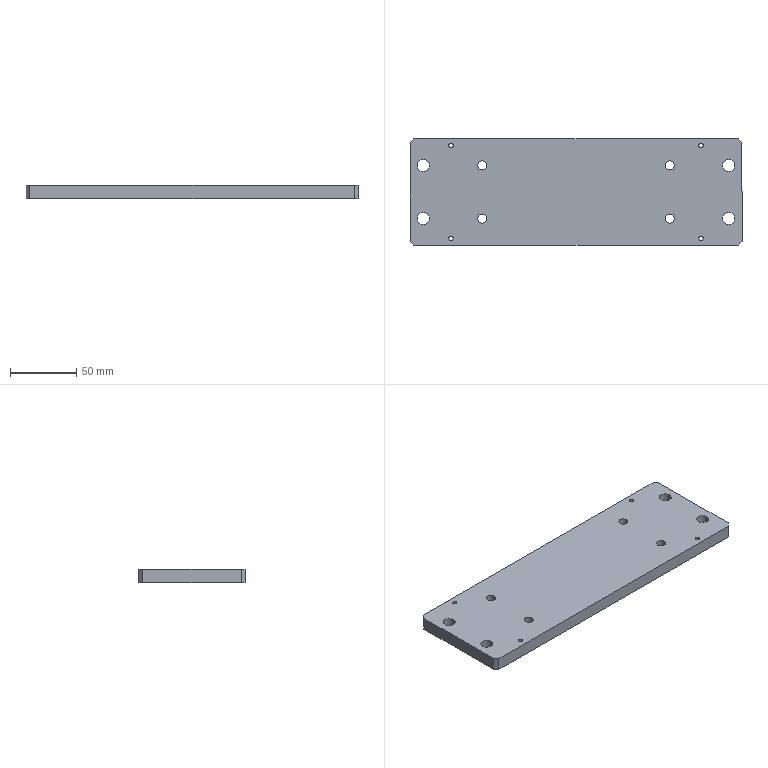Part | SolidWorks | features HoleWzd 3, MirrorPattern 3, Chamfer 1, Extrusion 1 | 1 solid | 34 faces | box 250 x 80 x 10 mm | volume 195481 mm3 | cylinder 24 | plane 10 | commonest cylinder face diameters 3.3 x8 6.8 x8 9 x8
STEP:
#1=CARTESIAN_POINT('',(92.472,75.,0.));
#2=VERTEX_POINT('',#1);
#3=CARTESIAN_POINT('',(95.772,75.,0.));
#4=VERTEX_POINT('',#3);
#5=CARTESIAN_POINT('',(94.122,75.,0.));
#6=DIRECTION('',(0.,0.,1.));
#7=DIRECTION('',(1.,0.,0.));
#8=AXIS2_PLACEMENT_3D('',#5,#6,#7);
#9=CIRCLE('',#8,1.65);
#10=EDGE_CURVE('',#2,#4,#9,.T.);
#11=ORIENTED_EDGE('',*,*,#10,.F.);
#12=CARTESIAN_POINT('',(92.472,75.,10.));
#13=VERTEX_POINT('',#12);
#14=CARTESIAN_POINT('',(92.472,75.,10.));
#15=DIRECTION('',(0.,0.,1.));
#16=VECTOR('',#15,1000.);
#17=LINE('',#14,#16);
#18=EDGE_CURVE('',#2,#13,#17,.T.);
#19=ORIENTED_EDGE('',*,*,#18,.T.);
#20=CARTESIAN_POINT('',(95.772,75.,10.));
#21=VERTEX_POINT('',#20);
#22=CARTESIAN_POINT('',(94.122,75.,10.));
#23=DIRECTION('',(0.,0.,1.));
#24=DIRECTION('',(1.,0.,0.));
#25=AXIS2_PLACEMENT_3D('',#22,#23,#24);
#26=CIRCLE('',#25,1.65);
#27=EDGE_CURVE('',#13,#21,#26,.T.);
#28=ORIENTED_EDGE('',*,*,#27,.T.);
#29=CARTESIAN_POINT('',(95.772,75.,10.));
#30=DIRECTION('',(0.,0.,1.));
#31=VECTOR('',#30,1000.);
#32=LINE('',#29,#31);
#33=EDGE_CURVE('',#4,#21,#32,.T.);
#34=ORIENTED_EDGE('',*,*,#33,.F.);
#35=EDGE_LOOP('',(#11,#19,#28,#34));
#36=FACE_OUTER_BOUND('',#35,.T.);
#37=CARTESIAN_POINT('',(94.122,75.,10.));
#38=DIRECTION('',(0.,0.,1.));
#39=DIRECTION('',(1.,0.,0.));
#40=AXIS2_PLACEMENT_3D('',#37,#38,#39);
#41=CYLINDRICAL_SURFACE('',#40,1.65);
#42=ADVANCED_FACE('',(#36),#41,.F.);
#43=CARTESIAN_POINT('',(92.472,5.,0.));
#44=VERTEX_POINT('',#43);
#45=CARTESIAN_POINT('',(95.772,5.,0.));
#46=VERTEX_POINT('',#45);
#47=CARTESIAN_POINT('',(94.122,5.,0.));
#48=DIRECTION('',(0.,0.,1.));
#49=DIRECTION('',(1.,0.,0.));
#50=AXIS2_PLACEMENT_3D('',#47,#48,#49);
#51=CIRCLE('',#50,1.65);
#52=EDGE_CURVE('',#44,#46,#51,.T.);
#53=ORIENTED_EDGE('',*,*,#52,.F.);
#54=CARTESIAN_POINT('',(92.472,5.,10.));
#55=VERTEX_POINT('',#54);
#56=CARTESIAN_POINT('',(92.472,5.,10.));
#57=DIRECTION('',(0.,0.,1.));
#58=VECTOR('',#57,1000.);
#59=LINE('',#56,#58);
#60=EDGE_CURVE('',#44,#55,#59,.T.);
#61=ORIENTED_EDGE('',*,*,#60,.T.);
#62=CARTESIAN_POINT('',(95.772,5.,10.));
#63=VERTEX_POINT('',#62);
#64=CARTESIAN_POINT('',(94.122,5.,10.));
#65=DIRECTION('',(0.,0.,1.));
#66=DIRECTION('',(1.,0.,0.));
#67=AXIS2_PLACEMENT_3D('',#64,#65,#66);
#68=CIRCLE('',#67,1.65);
#69=EDGE_CURVE('',#55,#63,#68,.T.);
#70=ORIENTED_EDGE('',*,*,#69,.T.);
#71=CARTESIAN_POINT('',(95.772,5.,10.));
#72=DIRECTION('',(0.,0.,1.));
#73=VECTOR('',#72,1000.);
#74=LINE('',#71,#73);
#75=EDGE_CURVE('',#46,#63,#74,.T.);
#76=ORIENTED_EDGE('',*,*,#75,.F.);
#77=EDGE_LOOP('',(#53,#61,#70,#76));
#78=FACE_OUTER_BOUND('',#77,.T.);
#79=CARTESIAN_POINT('',(94.122,5.,10.));
#80=DIRECTION('',(0.,0.,1.));
#81=DIRECTION('',(1.,0.,0.));
#82=AXIS2_PLACEMENT_3D('',#79,#80,#81);
#83=CYLINDRICAL_SURFACE('',#82,1.65);
#84=ADVANCED_FACE('',(#78),#83,.F.);
#85=CARTESIAN_POINT('',(-95.772,75.,0.));
#86=VERTEX_POINT('',#85);
#87=CARTESIAN_POINT('',(-92.472,75.,0.));
#88=VERTEX_POINT('',#87);
#89=CARTESIAN_POINT('',(-94.122,75.,0.));
#90=DIRECTION('',(0.,0.,1.));
#91=DIRECTION('',(1.,0.,0.));
#92=AXIS2_PLACEMENT_3D('',#89,#90,#91);
#93=CIRCLE('',#92,1.65);
#94=EDGE_CURVE('',#86,#88,#93,.T.);
#95=ORIENTED_EDGE('',*,*,#94,.F.);
#96=CARTESIAN_POINT('',(-95.772,75.,10.));
#97=VERTEX_POINT('',#96);
#98=CARTESIAN_POINT('',(-95.772,75.,10.));
#99=DIRECTION('',(0.,0.,1.));
#100=VECTOR('',#99,1000.);
#101=LINE('',#98,#100);
#102=EDGE_CURVE('',#86,#97,#101,.T.);
#103=ORIENTED_EDGE('',*,*,#102,.T.);
#104=CARTESIAN_POINT('',(-92.472,75.,10.));
#105=VERTEX_POINT('',#104);
#106=CARTESIAN_POINT('',(-94.122,75.,10.));
#107=DIRECTION('',(0.,0.,1.));
#108=DIRECTION('',(1.,0.,0.));
#109=AXIS2_PLACEMENT_3D('',#106,#107,#108);
#110=CIRCLE('',#109,1.65);
#111=EDGE_CURVE('',#97,#105,#110,.T.);
#112=ORIENTED_EDGE('',*,*,#111,.T.);
#113=CARTESIAN_POINT('',(-92.472,75.,10.));
#114=DIRECTION('',(0.,0.,1.));
#115=VECTOR('',#114,1000.);
#116=LINE('',#113,#115);
#117=EDGE_CURVE('',#88,#105,#116,.T.);
#118=ORIENTED_EDGE('',*,*,#117,.F.);
#119=EDGE_LOOP('',(#95,#103,#112,#118));
#120=FACE_OUTER_BOUND('',#119,.T.);
#121=CARTESIAN_POINT('',(-94.122,75.,10.));
#122=DIRECTION('',(0.,0.,1.));
#123=DIRECTION('',(1.,0.,0.));
#124=AXIS2_PLACEMENT_3D('',#121,#122,#123);
#125=CYLINDRICAL_SURFACE('',#124,1.65);
#126=ADVANCED_FACE('',(#120),#125,.F.);
#127=CARTESIAN_POINT('',(-95.772,5.,0.));
#128=VERTEX_POINT('',#127);
#129=CARTESIAN_POINT('',(-92.472,5.,0.));
#130=VERTEX_POINT('',#129);
#131=CARTESIAN_POINT('',(-94.122,5.,0.));
#132=DIRECTION('',(0.,0.,1.));
#133=DIRECTION('',(1.,0.,0.));
#134=AXIS2_PLACEMENT_3D('',#131,#132,#133);
#135=CIRCLE('',#134,1.65);
#136=EDGE_CURVE('',#128,#130,#135,.T.);
#137=ORIENTED_EDGE('',*,*,#136,.F.);
#138=CARTESIAN_POINT('',(-95.772,5.,10.));
#139=VERTEX_POINT('',#138);
#140=CARTESIAN_POINT('',(-95.772,5.,10.));
#141=DIRECTION('',(0.,0.,1.));
#142=VECTOR('',#141,1000.);
#143=LINE('',#140,#142);
#144=EDGE_CURVE('',#128,#139,#143,.T.);
#145=ORIENTED_EDGE('',*,*,#144,.T.);
#146=CARTESIAN_POINT('',(-92.472,5.,10.));
#147=VERTEX_POINT('',#146);
#148=CARTESIAN_POINT('',(-94.122,5.,10.));
#149=DIRECTION('',(0.,0.,1.));
#150=DIRECTION('',(1.,0.,0.));
#151=AXIS2_PLACEMENT_3D('',#148,#149,#150);
#152=CIRCLE('',#151,1.65);
#153=EDGE_CURVE('',#139,#147,#152,.T.);
#154=ORIENTED_EDGE('',*,*,#153,.T.);
#155=CARTESIAN_POINT('',(-92.472,5.,10.));
#156=DIRECTION('',(0.,0.,1.));
#157=VECTOR('',#156,1000.);
#158=LINE('',#155,#157);
#159=EDGE_CURVE('',#130,#147,#158,.T.);
#160=ORIENTED_EDGE('',*,*,#159,.F.);
#161=EDGE_LOOP('',(#137,#145,#154,#160));
#162=FACE_OUTER_BOUND('',#161,.T.);
#163=CARTESIAN_POINT('',(-94.122,5.,10.));
#164=DIRECTION('',(0.,0.,1.));
#165=DIRECTION('',(1.,0.,0.));
#166=AXIS2_PLACEMENT_3D('',#163,#164,#165);
#167=CYLINDRICAL_SURFACE('',#166,1.65);
#168=ADVANCED_FACE('',(#162),#167,.F.);
#169=CARTESIAN_POINT('',(-73.9,60.,0.));
#170=VERTEX_POINT('',#169);
#171=CARTESIAN_POINT('',(-67.1,60.,0.));
#172=VERTEX_POINT('',#171);
#173=CARTESIAN_POINT('',(-70.5,60.,0.));
#174=DIRECTION('',(0.,0.,1.));
#175=DIRECTION('',(1.,0.,0.));
#176=AXIS2_PLACEMENT_3D('',#173,#174,#175);
#177=CIRCLE('',#176,3.4);
#178=EDGE_CURVE('',#170,#172,#177,.T.);
#179=ORIENTED_EDGE('',*,*,#178,.F.);
#180=CARTESIAN_POINT('',(-73.9,60.,10.));
#181=VERTEX_POINT('',#180);
#182=CARTESIAN_POINT('',(-73.9,60.,10.));
#183=DIRECTION('',(0.,0.,1.));
#184=VECTOR('',#183,1000.);
#185=LINE('',#182,#184);
#186=EDGE_CURVE('',#170,#181,#185,.T.);
#187=ORIENTED_EDGE('',*,*,#186,.T.);
#188=CARTESIAN_POINT('',(-67.1,60.,10.));
#189=VERTEX_POINT('',#188);
#190=CARTESIAN_POINT('',(-70.5,60.,10.));
#191=DIRECTION('',(0.,0.,1.));
#192=DIRECTION('',(1.,0.,0.));
#193=AXIS2_PLACEMENT_3D('',#190,#191,#192);
#194=CIRCLE('',#193,3.4);
#195=EDGE_CURVE('',#181,#189,#194,.T.);
#196=ORIENTED_EDGE('',*,*,#195,.T.);
#197=CARTESIAN_POINT('',(-67.1,60.,10.));
#198=DIRECTION('',(0.,0.,1.));
#199=VECTOR('',#198,1000.);
#200=LINE('',#197,#199);
#201=EDGE_CURVE('',#172,#189,#200,.T.);
#202=ORIENTED_EDGE('',*,*,#201,.F.);
#203=EDGE_LOOP('',(#179,#187,#196,#202));
#204=FACE_OUTER_BOUND('',#203,.T.);
#205=CARTESIAN_POINT('',(-70.5,60.,10.));
#206=DIRECTION('',(0.,0.,1.));
#207=DIRECTION('',(1.,0.,0.));
#208=AXIS2_PLACEMENT_3D('',#205,#206,#207);
#209=CYLINDRICAL_SURFACE('',#208,3.4);
#210=ADVANCED_FACE('',(#204),#209,.F.);
#211=CARTESIAN_POINT('',(-73.9,20.,0.));
#212=VERTEX_POINT('',#211);
#213=CARTESIAN_POINT('',(-67.1,20.,0.));
#214=VERTEX_POINT('',#213);
#215=CARTESIAN_POINT('',(-70.5,20.,0.));
#216=DIRECTION('',(0.,0.,1.));
#217=DIRECTION('',(1.,0.,0.));
#218=AXIS2_PLACEMENT_3D('',#215,#216,#217);
#219=CIRCLE('',#218,3.4);
#220=EDGE_CURVE('',#212,#214,#219,.T.);
#221=ORIENTED_EDGE('',*,*,#220,.F.);
#222=CARTESIAN_POINT('',(-73.9,20.,10.));
#223=VERTEX_POINT('',#222);
#224=CARTESIAN_POINT('',(-73.9,20.,10.));
#225=DIRECTION('',(0.,0.,1.));
#226=VECTOR('',#225,1000.);
#227=LINE('',#224,#226);
#228=EDGE_CURVE('',#212,#223,#227,.T.);
#229=ORIENTED_EDGE('',*,*,#228,.T.);
#230=CARTESIAN_POINT('',(-67.1,20.,10.));
#231=VERTEX_POINT('',#230);
#232=CARTESIAN_POINT('',(-70.5,20.,10.));
#233=DIRECTION('',(0.,0.,1.));
#234=DIRECTION('',(1.,0.,0.));
#235=AXIS2_PLACEMENT_3D('',#232,#233,#234);
#236=CIRCLE('',#235,3.4);
#237=EDGE_CURVE('',#223,#231,#236,.T.);
#238=ORIENTED_EDGE('',*,*,#237,.T.);
#239=CARTESIAN_POINT('',(-67.1,20.,10.));
#240=DIRECTION('',(0.,0.,1.));
#241=VECTOR('',#240,1000.);
#242=LINE('',#239,#241);
#243=EDGE_CURVE('',#214,#231,#242,.T.);
#244=ORIENTED_EDGE('',*,*,#243,.F.);
#245=EDGE_LOOP('',(#221,#229,#238,#244));
#246=FACE_OUTER_BOUND('',#245,.T.);
#247=CARTESIAN_POINT('',(-70.5,20.,10.));
#248=DIRECTION('',(0.,0.,1.));
#249=DIRECTION('',(1.,0.,0.));
#250=AXIS2_PLACEMENT_3D('',#247,#248,#249);
#251=CYLINDRICAL_SURFACE('',#250,3.4);
#252=ADVANCED_FACE('',(#246),#251,.F.);
#253=CARTESIAN_POINT('',(67.1,60.,0.));
#254=VERTEX_POINT('',#253);
#255=CARTESIAN_POINT('',(73.9,60.,0.));
#256=VERTEX_POINT('',#255);
#257=CARTESIAN_POINT('',(70.5,60.,0.));
#258=DIRECTION('',(0.,0.,1.));
#259=DIRECTION('',(1.,0.,0.));
#260=AXIS2_PLACEMENT_3D('',#257,#258,#259);
#261=CIRCLE('',#260,3.4);
#262=EDGE_CURVE('',#254,#256,#261,.T.);
#263=ORIENTED_EDGE('',*,*,#262,.F.);
#264=CARTESIAN_POINT('',(67.1,60.,10.));
#265=VERTEX_POINT('',#264);
#266=CARTESIAN_POINT('',(67.1,60.,10.));
#267=DIRECTION('',(0.,0.,1.));
#268=VECTOR('',#267,1000.);
#269=LINE('',#266,#268);
#270=EDGE_CURVE('',#254,#265,#269,.T.);
#271=ORIENTED_EDGE('',*,*,#270,.T.);
#272=CARTESIAN_POINT('',(73.9,60.,10.));
#273=VERTEX_POINT('',#272);
#274=CARTESIAN_POINT('',(70.5,60.,10.));
#275=DIRECTION('',(0.,0.,1.));
#276=DIRECTION('',(1.,0.,0.));
#277=AXIS2_PLACEMENT_3D('',#274,#275,#276);
#278=CIRCLE('',#277,3.4);
#279=EDGE_CURVE('',#265,#273,#278,.T.);
#280=ORIENTED_EDGE('',*,*,#279,.T.);
#281=CARTESIAN_POINT('',(73.9,60.,10.));
#282=DIRECTION('',(0.,0.,1.));
#283=VECTOR('',#282,1000.);
#284=LINE('',#281,#283);
#285=EDGE_CURVE('',#256,#273,#284,.T.);
#286=ORIENTED_EDGE('',*,*,#285,.F.);
#287=EDGE_LOOP('',(#263,#271,#280,#286));
#288=FACE_OUTER_BOUND('',#287,.T.);
#289=CARTESIAN_POINT('',(70.5,60.,10.));
#290=DIRECTION('',(0.,0.,1.));
#291=DIRECTION('',(1.,0.,0.));
#292=AXIS2_PLACEMENT_3D('',#289,#290,#291);
#293=CYLINDRICAL_SURFACE('',#292,3.4);
#294=ADVANCED_FACE('',(#288),#293,.F.);
#295=CARTESIAN_POINT('',(67.1,20.,0.));
#296=VERTEX_POINT('',#295);
#297=CARTESIAN_POINT('',(73.9,20.,0.));
#298=VERTEX_POINT('',#297);
#299=CARTESIAN_POINT('',(70.5,20.,0.));
#300=DIRECTION('',(0.,0.,1.));
#301=DIRECTION('',(1.,0.,0.));
#302=AXIS2_PLACEMENT_3D('',#299,#300,#301);
#303=CIRCLE('',#302,3.4);
#304=EDGE_CURVE('',#296,#298,#303,.T.);
#305=ORIENTED_EDGE('',*,*,#304,.F.);
#306=CARTESIAN_POINT('',(67.1,20.,10.));
#307=VERTEX_POINT('',#306);
#308=CARTESIAN_POINT('',(67.1,20.,10.));
#309=DIRECTION('',(0.,0.,1.));
#310=VECTOR('',#309,1000.);
#311=LINE('',#308,#310);
#312=EDGE_CURVE('',#296,#307,#311,.T.);
#313=ORIENTED_EDGE('',*,*,#312,.T.);
#314=CARTESIAN_POINT('',(73.9,20.,10.));
#315=VERTEX_POINT('',#314);
#316=CARTESIAN_POINT('',(70.5,20.,10.));
#317=DIRECTION('',(0.,0.,1.));
#318=DIRECTION('',(1.,0.,0.));
#319=AXIS2_PLACEMENT_3D('',#316,#317,#318);
#320=CIRCLE('',#319,3.4);
#321=EDGE_CURVE('',#307,#315,#320,.T.);
#322=ORIENTED_EDGE('',*,*,#321,.T.);
#323=CARTESIAN_POINT('',(73.9,20.,10.));
#324=DIRECTION('',(0.,0.,1.));
#325=VECTOR('',#324,1000.);
#326=LINE('',#323,#325);
#327=EDGE_CURVE('',#298,#315,#326,.T.);
#328=ORIENTED_EDGE('',*,*,#327,.F.);
#329=EDGE_LOOP('',(#305,#313,#322,#328));
#330=FACE_OUTER_BOUND('',#329,.T.);
#331=CARTESIAN_POINT('',(70.5,20.,10.));
#332=DIRECTION('',(0.,0.,1.));
#333=DIRECTION('',(1.,0.,0.));
#334=AXIS2_PLACEMENT_3D('',#331,#332,#333);
#335=CYLINDRICAL_SURFACE('',#334,3.4);
#336=ADVANCED_FACE('',(#330),#335,.F.);
#337=CARTESIAN_POINT('',(-119.5,20.,0.));
#338=VERTEX_POINT('',#337);
#339=CARTESIAN_POINT('',(-110.5,20.,0.));
#340=VERTEX_POINT('',#339);
#341=CARTESIAN_POINT('',(-115.,20.,0.));
#342=DIRECTION('',(0.,0.,1.));
#343=DIRECTION('',(1.,0.,0.));
#344=AXIS2_PLACEMENT_3D('',#341,#342,#343);
#345=CIRCLE('',#344,4.5);
#346=EDGE_CURVE('',#338,#340,#345,.T.);
#347=ORIENTED_EDGE('',*,*,#346,.F.);
#348=CARTESIAN_POINT('',(-119.5,20.,10.));
#349=VERTEX_POINT('',#348);
#350=CARTESIAN_POINT('',(-119.5,20.,10.));
#351=DIRECTION('',(0.,0.,1.));
#352=VECTOR('',#351,1000.);
#353=LINE('',#350,#352);
#354=EDGE_CURVE('',#338,#349,#353,.T.);
#355=ORIENTED_EDGE('',*,*,#354,.T.);
#356=CARTESIAN_POINT('',(-110.5,20.,10.));
#357=VERTEX_POINT('',#356);
#358=CARTESIAN_POINT('',(-115.,20.,10.));
#359=DIRECTION('',(0.,0.,1.));
#360=DIRECTION('',(1.,0.,0.));
#361=AXIS2_PLACEMENT_3D('',#358,#359,#360);
#362=CIRCLE('',#361,4.5);
#363=EDGE_CURVE('',#349,#357,#362,.T.);
#364=ORIENTED_EDGE('',*,*,#363,.T.);
#365=CARTESIAN_POINT('',(-110.5,20.,10.));
#366=DIRECTION('',(0.,0.,1.));
#367=VECTOR('',#366,1000.);
#368=LINE('',#365,#367);
#369=EDGE_CURVE('',#340,#357,#368,.T.);
#370=ORIENTED_EDGE('',*,*,#369,.F.);
#371=EDGE_LOOP('',(#347,#355,#364,#370));
#372=FACE_OUTER_BOUND('',#371,.T.);
#373=CARTESIAN_POINT('',(-115.,20.,10.));
#374=DIRECTION('',(0.,0.,1.));
#375=DIRECTION('',(1.,0.,0.));
#376=AXIS2_PLACEMENT_3D('',#373,#374,#375);
#377=CYLINDRICAL_SURFACE('',#376,4.5);
#378=ADVANCED_FACE('',(#372),#377,.F.);
#379=CARTESIAN_POINT('',(-119.5,60.,0.));
#380=VERTEX_POINT('',#379);
#381=CARTESIAN_POINT('',(-110.5,60.,0.));
#382=VERTEX_POINT('',#381);
#383=CARTESIAN_POINT('',(-115.,60.,0.));
#384=DIRECTION('',(0.,0.,1.));
#385=DIRECTION('',(1.,0.,0.));
#386=AXIS2_PLACEMENT_3D('',#383,#384,#385);
#387=CIRCLE('',#386,4.5);
#388=EDGE_CURVE('',#380,#382,#387,.T.);
#389=ORIENTED_EDGE('',*,*,#388,.F.);
#390=CARTESIAN_POINT('',(-119.5,60.,10.));
#391=VERTEX_POINT('',#390);
#392=CARTESIAN_POINT('',(-119.5,60.,10.));
#393=DIRECTION('',(0.,0.,1.));
#394=VECTOR('',#393,1000.);
#395=LINE('',#392,#394);
#396=EDGE_CURVE('',#380,#391,#395,.T.);
#397=ORIENTED_EDGE('',*,*,#396,.T.);
#398=CARTESIAN_POINT('',(-110.5,60.,10.));
#399=VERTEX_POINT('',#398);
#400=CARTESIAN_POINT('',(-115.,60.,10.));
#401=DIRECTION('',(0.,0.,1.));
#402=DIRECTION('',(1.,0.,0.));
#403=AXIS2_PLACEMENT_3D('',#400,#401,#402);
#404=CIRCLE('',#403,4.5);
#405=EDGE_CURVE('',#391,#399,#404,.T.);
#406=ORIENTED_EDGE('',*,*,#405,.T.);
#407=CARTESIAN_POINT('',(-110.5,60.,10.));
#408=DIRECTION('',(0.,0.,1.));
#409=VECTOR('',#408,1000.);
#410=LINE('',#407,#409);
#411=EDGE_CURVE('',#382,#399,#410,.T.);
#412=ORIENTED_EDGE('',*,*,#411,.F.);
#413=EDGE_LOOP('',(#389,#397,#406,#412));
#414=FACE_OUTER_BOUND('',#413,.T.);
#415=CARTESIAN_POINT('',(-115.,60.,10.));
#416=DIRECTION('',(0.,0.,1.));
#417=DIRECTION('',(1.,0.,0.));
#418=AXIS2_PLACEMENT_3D('',#415,#416,#417);
#419=CYLINDRICAL_SURFACE('',#418,4.5);
#420=ADVANCED_FACE('',(#414),#419,.F.);
#421=CARTESIAN_POINT('',(110.5,20.,0.));
#422=VERTEX_POINT('',#421);
#423=CARTESIAN_POINT('',(119.5,20.,0.));
#424=VERTEX_POINT('',#423);
#425=CARTESIAN_POINT('',(115.,20.,0.));
#426=DIRECTION('',(0.,0.,1.));
#427=DIRECTION('',(1.,0.,0.));
#428=AXIS2_PLACEMENT_3D('',#425,#426,#427);
#429=CIRCLE('',#428,4.5);
#430=EDGE_CURVE('',#422,#424,#429,.T.);
#431=ORIENTED_EDGE('',*,*,#430,.F.);
#432=CARTESIAN_POINT('',(110.5,20.,10.));
#433=VERTEX_POINT('',#432);
#434=CARTESIAN_POINT('',(110.5,20.,10.));
#435=DIRECTION('',(0.,0.,1.));
#436=VECTOR('',#435,1000.);
#437=LINE('',#434,#436);
#438=EDGE_CURVE('',#422,#433,#437,.T.);
#439=ORIENTED_EDGE('',*,*,#438,.T.);
#440=CARTESIAN_POINT('',(119.5,20.,10.));
#441=VERTEX_POINT('',#440);
#442=CARTESIAN_POINT('',(115.,20.,10.));
#443=DIRECTION('',(0.,0.,1.));
#444=DIRECTION('',(1.,0.,0.));
#445=AXIS2_PLACEMENT_3D('',#442,#443,#444);
#446=CIRCLE('',#445,4.5);
#447=EDGE_CURVE('',#433,#441,#446,.T.);
#448=ORIENTED_EDGE('',*,*,#447,.T.);
#449=CARTESIAN_POINT('',(119.5,20.,10.));
#450=DIRECTION('',(0.,0.,1.));
#451=VECTOR('',#450,1000.);
#452=LINE('',#449,#451);
#453=EDGE_CURVE('',#424,#441,#452,.T.);
#454=ORIENTED_EDGE('',*,*,#453,.F.);
#455=EDGE_LOOP('',(#431,#439,#448,#454));
#456=FACE_OUTER_BOUND('',#455,.T.);
#457=CARTESIAN_POINT('',(115.,20.,10.));
#458=DIRECTION('',(0.,0.,1.));
#459=DIRECTION('',(1.,0.,0.));
#460=AXIS2_PLACEMENT_3D('',#457,#458,#459);
#461=CYLINDRICAL_SURFACE('',#460,4.5);
#462=ADVANCED_FACE('',(#456),#461,.F.);
#463=CARTESIAN_POINT('',(110.5,60.,0.));
#464=VERTEX_POINT('',#463);
#465=CARTESIAN_POINT('',(119.5,60.,0.));
#466=VERTEX_POINT('',#465);
#467=CARTESIAN_POINT('',(115.,60.,0.));
#468=DIRECTION('',(0.,0.,1.));
#469=DIRECTION('',(1.,0.,0.));
#470=AXIS2_PLACEMENT_3D('',#467,#468,#469);
#471=CIRCLE('',#470,4.5);
#472=EDGE_CURVE('',#464,#466,#471,.T.);
#473=ORIENTED_EDGE('',*,*,#472,.F.);
#474=CARTESIAN_POINT('',(110.5,60.,10.));
#475=VERTEX_POINT('',#474);
#476=CARTESIAN_POINT('',(110.5,60.,10.));
#477=DIRECTION('',(0.,0.,1.));
#478=VECTOR('',#477,1000.);
#479=LINE('',#476,#478);
#480=EDGE_CURVE('',#464,#475,#479,.T.);
#481=ORIENTED_EDGE('',*,*,#480,.T.);
#482=CARTESIAN_POINT('',(119.5,60.,10.));
#483=VERTEX_POINT('',#482);
#484=CARTESIAN_POINT('',(115.,60.,10.));
#485=DIRECTION('',(0.,0.,1.));
#486=DIRECTION('',(1.,0.,0.));
#487=AXIS2_PLACEMENT_3D('',#484,#485,#486);
#488=CIRCLE('',#487,4.5);
#489=EDGE_CURVE('',#475,#483,#488,.T.);
#490=ORIENTED_EDGE('',*,*,#489,.T.);
#491=CARTESIAN_POINT('',(119.5,60.,10.));
#492=DIRECTION('',(0.,0.,1.));
#493=VECTOR('',#492,1000.);
#494=LINE('',#491,#493);
#495=EDGE_CURVE('',#466,#483,#494,.T.);
#496=ORIENTED_EDGE('',*,*,#495,.F.);
#497=EDGE_LOOP('',(#473,#481,#490,#496));
#498=FACE_OUTER_BOUND('',#497,.T.);
#499=CARTESIAN_POINT('',(115.,60.,10.));
#500=DIRECTION('',(0.,0.,1.));
#501=DIRECTION('',(1.,0.,0.));
#502=AXIS2_PLACEMENT_3D('',#499,#500,#501);
#503=CYLINDRICAL_SURFACE('',#502,4.5);
#504=ADVANCED_FACE('',(#498),#503,.F.);
#505=CARTESIAN_POINT('',(-125.,77.,10.));
#506=VERTEX_POINT('',#505);
#507=CARTESIAN_POINT('',(-125.,3.,10.));
#508=VERTEX_POINT('',#507);
#509=CARTESIAN_POINT('',(-125.,80.,10.));
#510=DIRECTION('',(0.,-1.,0.));
#511=VECTOR('',#510,1000.);
#512=LINE('',#509,#511);
#513=EDGE_CURVE('',#506,#508,#512,.T.);
#514=ORIENTED_EDGE('',*,*,#513,.F.);
#515=CARTESIAN_POINT('',(-125.,77.,0.));
#516=VERTEX_POINT('',#515);
#517=CARTESIAN_POINT('',(-125.,77.,10.));
#518=DIRECTION('',(0.,0.,-1.));
#519=VECTOR('',#518,1000.);
#520=LINE('',#517,#519);
#521=EDGE_CURVE('',#506,#516,#520,.T.);
#522=ORIENTED_EDGE('',*,*,#521,.T.);
#523=CARTESIAN_POINT('',(-125.,3.,0.));
#524=VERTEX_POINT('',#523);
#525=CARTESIAN_POINT('',(-125.,80.,0.));
#526=DIRECTION('',(0.,-1.,0.));
#527=VECTOR('',#526,1000.);
#528=LINE('',#525,#527);
#529=EDGE_CURVE('',#516,#524,#528,.T.);
#530=ORIENTED_EDGE('',*,*,#529,.T.);
#531=CARTESIAN_POINT('',(-125.,3.,10.));
#532=DIRECTION('',(0.,0.,1.));
#533=VECTOR('',#532,1000.);
#534=LINE('',#531,#533);
#535=EDGE_CURVE('',#524,#508,#534,.T.);
#536=ORIENTED_EDGE('',*,*,#535,.T.);
#537=EDGE_LOOP('',(#514,#522,#530,#536));
#538=FACE_OUTER_BOUND('',#537,.T.);
#539=CARTESIAN_POINT('',(-125.,80.,10.));
#540=DIRECTION('',(1.,0.,0.));
#541=DIRECTION('',(0.,1.,0.));
#542=AXIS2_PLACEMENT_3D('',#539,#540,#541);
#543=PLANE('',#542);
#544=ADVANCED_FACE('',(#538),#543,.F.);
#545=CARTESIAN_POINT('',(-122.,0.,10.));
#546=VERTEX_POINT('',#545);
#547=CARTESIAN_POINT('',(122.,0.,10.));
#548=VERTEX_POINT('',#547);
#549=CARTESIAN_POINT('',(-125.,0.,10.));
#550=DIRECTION('',(1.,0.,0.));
#551=VECTOR('',#550,1000.);
#552=LINE('',#549,#551);
#553=EDGE_CURVE('',#546,#548,#552,.T.);
#554=ORIENTED_EDGE('',*,*,#553,.F.);
#555=CARTESIAN_POINT('',(-122.,0.,0.));
#556=VERTEX_POINT('',#555);
#557=CARTESIAN_POINT('',(-122.,0.,10.));
#558=DIRECTION('',(0.,0.,-1.));
#559=VECTOR('',#558,1000.);
#560=LINE('',#557,#559);
#561=EDGE_CURVE('',#546,#556,#560,.T.);
#562=ORIENTED_EDGE('',*,*,#561,.T.);
#563=CARTESIAN_POINT('',(122.,0.,0.));
#564=VERTEX_POINT('',#563);
#565=CARTESIAN_POINT('',(-125.,0.,0.));
#566=DIRECTION('',(1.,0.,0.));
#567=VECTOR('',#566,1000.);
#568=LINE('',#565,#567);
#569=EDGE_CURVE('',#556,#564,#568,.T.);
#570=ORIENTED_EDGE('',*,*,#569,.T.);
#571=CARTESIAN_POINT('',(122.,0.,10.));
#572=DIRECTION('',(0.,0.,1.));
#573=VECTOR('',#572,1000.);
#574=LINE('',#571,#573);
#575=EDGE_CURVE('',#564,#548,#574,.T.);
#576=ORIENTED_EDGE('',*,*,#575,.T.);
#577=EDGE_LOOP('',(#554,#562,#570,#576));
#578=FACE_OUTER_BOUND('',#577,.T.);
#579=CARTESIAN_POINT('',(-125.,0.,10.));
#580=DIRECTION('',(0.,1.,0.));
#581=DIRECTION('',(0.,0.,1.));
#582=AXIS2_PLACEMENT_3D('',#579,#580,#581);
#583=PLANE('',#582);
#584=ADVANCED_FACE('',(#578),#583,.F.);
#585=CARTESIAN_POINT('',(125.,3.,10.));
#586=VERTEX_POINT('',#585);
#587=CARTESIAN_POINT('',(125.,77.,10.));
#588=VERTEX_POINT('',#587);
#589=CARTESIAN_POINT('',(125.,80.,10.));
#590=DIRECTION('',(0.,1.,0.));
#591=VECTOR('',#590,1000.);
#592=LINE('',#589,#591);
#593=EDGE_CURVE('',#586,#588,#592,.T.);
#594=ORIENTED_EDGE('',*,*,#593,.F.);
#595=CARTESIAN_POINT('',(125.,3.,0.));
#596=VERTEX_POINT('',#595);
#597=CARTESIAN_POINT('',(125.,3.,10.));
#598=DIRECTION('',(0.,0.,-1.));
#599=VECTOR('',#598,1000.);
#600=LINE('',#597,#599);
#601=EDGE_CURVE('',#586,#596,#600,.T.);
#602=ORIENTED_EDGE('',*,*,#601,.T.);
#603=CARTESIAN_POINT('',(125.,77.,0.));
#604=VERTEX_POINT('',#603);
#605=CARTESIAN_POINT('',(125.,80.,0.));
#606=DIRECTION('',(0.,1.,0.));
#607=VECTOR('',#606,1000.);
#608=LINE('',#605,#607);
#609=EDGE_CURVE('',#596,#604,#608,.T.);
#610=ORIENTED_EDGE('',*,*,#609,.T.);
#611=CARTESIAN_POINT('',(125.,77.,10.));
#612=DIRECTION('',(0.,0.,1.));
#613=VECTOR('',#612,1000.);
#614=LINE('',#611,#613);
#615=EDGE_CURVE('',#604,#588,#614,.T.);
#616=ORIENTED_EDGE('',*,*,#615,.T.);
#617=EDGE_LOOP('',(#594,#602,#610,#616));
#618=FACE_OUTER_BOUND('',#617,.T.);
#619=CARTESIAN_POINT('',(125.,80.,10.));
#620=DIRECTION('',(-1.,0.,0.));
#621=DIRECTION('',(0.,-1.,0.));
#622=AXIS2_PLACEMENT_3D('',#619,#620,#621);
#623=PLANE('',#622);
#624=ADVANCED_FACE('',(#618),#623,.F.);
#625=CARTESIAN_POINT('',(122.,80.,0.));
#626=VERTEX_POINT('',#625);
#627=CARTESIAN_POINT('',(-122.,80.,0.));
#628=VERTEX_POINT('',#627);
#629=CARTESIAN_POINT('',(-125.,80.,0.));
#630=DIRECTION('',(-1.,0.,0.));
#631=VECTOR('',#630,1000.);
#632=LINE('',#629,#631);
#633=EDGE_CURVE('',#626,#628,#632,.T.);
#634=ORIENTED_EDGE('',*,*,#633,.T.);
#635=CARTESIAN_POINT('',(-122.,80.,10.));
#636=VERTEX_POINT('',#635);
#637=CARTESIAN_POINT('',(-122.,80.,10.));
#638=DIRECTION('',(0.,0.,1.));
#639=VECTOR('',#638,1000.);
#640=LINE('',#637,#639);
#641=EDGE_CURVE('',#628,#636,#640,.T.);
#642=ORIENTED_EDGE('',*,*,#641,.T.);
#643=CARTESIAN_POINT('',(122.,80.,10.));
#644=VERTEX_POINT('',#643);
#645=CARTESIAN_POINT('',(-125.,80.,10.));
#646=DIRECTION('',(-1.,0.,0.));
#647=VECTOR('',#646,1000.);
#648=LINE('',#645,#647);
#649=EDGE_CURVE('',#644,#636,#648,.T.);
#650=ORIENTED_EDGE('',*,*,#649,.F.);
#651=CARTESIAN_POINT('',(122.,80.,10.));
#652=DIRECTION('',(0.,0.,-1.));
#653=VECTOR('',#652,1000.);
#654=LINE('',#651,#653);
#655=EDGE_CURVE('',#644,#626,#654,.T.);
#656=ORIENTED_EDGE('',*,*,#655,.T.);
#657=EDGE_LOOP('',(#634,#642,#650,#656));
#658=FACE_OUTER_BOUND('',#657,.T.);
#659=CARTESIAN_POINT('',(-125.,80.,10.));
#660=DIRECTION('',(0.,-1.,0.));
#661=DIRECTION('',(0.,0.,-1.));
#662=AXIS2_PLACEMENT_3D('',#659,#660,#661);
#663=PLANE('',#662);
#664=ADVANCED_FACE('',(#658),#663,.F.);
#665=CARTESIAN_POINT('',(94.122,75.,10.));
#666=DIRECTION('',(0.,0.,1.));
#667=DIRECTION('',(1.,0.,0.));
#668=AXIS2_PLACEMENT_3D('',#665,#666,#667);
#669=CIRCLE('',#668,1.65);
#670=EDGE_CURVE('',#21,#13,#669,.T.);
#671=ORIENTED_EDGE('',*,*,#670,.F.);
#672=ORIENTED_EDGE('',*,*,#27,.F.);
#673=EDGE_LOOP('',(#671,#672));
#674=FACE_BOUND('',#673,.T.);
#675=CARTESIAN_POINT('',(94.122,5.,10.));
#676=DIRECTION('',(0.,0.,1.));
#677=DIRECTION('',(1.,0.,0.));
#678=AXIS2_PLACEMENT_3D('',#675,#676,#677);
#679=CIRCLE('',#678,1.65);
#680=EDGE_CURVE('',#63,#55,#679,.T.);
#681=ORIENTED_EDGE('',*,*,#680,.F.);
#682=ORIENTED_EDGE('',*,*,#69,.F.);
#683=EDGE_LOOP('',(#681,#682));
#684=FACE_BOUND('',#683,.T.);
#685=CARTESIAN_POINT('',(-94.122,75.,10.));
#686=DIRECTION('',(0.,0.,1.));
#687=DIRECTION('',(1.,0.,0.));
#688=AXIS2_PLACEMENT_3D('',#685,#686,#687);
#689=CIRCLE('',#688,1.65);
#690=EDGE_CURVE('',#105,#97,#689,.T.);
#691=ORIENTED_EDGE('',*,*,#690,.F.);
#692=ORIENTED_EDGE('',*,*,#111,.F.);
#693=EDGE_LOOP('',(#691,#692));
#694=FACE_BOUND('',#693,.T.);
#695=CARTESIAN_POINT('',(-94.122,5.,10.));
#696=DIRECTION('',(0.,0.,1.));
#697=DIRECTION('',(1.,0.,0.));
#698=AXIS2_PLACEMENT_3D('',#695,#696,#697);
#699=CIRCLE('',#698,1.65);
#700=EDGE_CURVE('',#147,#139,#699,.T.);
#701=ORIENTED_EDGE('',*,*,#700,.F.);
#702=ORIENTED_EDGE('',*,*,#153,.F.);
#703=EDGE_LOOP('',(#701,#702));
#704=FACE_BOUND('',#703,.T.);
#705=CARTESIAN_POINT('',(-70.5,60.,10.));
#706=DIRECTION('',(0.,0.,1.));
#707=DIRECTION('',(1.,0.,0.));
#708=AXIS2_PLACEMENT_3D('',#705,#706,#707);
#709=CIRCLE('',#708,3.4);
#710=EDGE_CURVE('',#189,#181,#709,.T.);
#711=ORIENTED_EDGE('',*,*,#710,.F.);
#712=ORIENTED_EDGE('',*,*,#195,.F.);
#713=EDGE_LOOP('',(#711,#712));
#714=FACE_BOUND('',#713,.T.);
#715=CARTESIAN_POINT('',(-70.5,20.,10.));
#716=DIRECTION('',(0.,0.,1.));
#717=DIRECTION('',(1.,0.,0.));
#718=AXIS2_PLACEMENT_3D('',#715,#716,#717);
#719=CIRCLE('',#718,3.4);
#720=EDGE_CURVE('',#231,#223,#719,.T.);
#721=ORIENTED_EDGE('',*,*,#720,.F.);
#722=ORIENTED_EDGE('',*,*,#237,.F.);
#723=EDGE_LOOP('',(#721,#722));
#724=FACE_BOUND('',#723,.T.);
#725=CARTESIAN_POINT('',(70.5,60.,10.));
#726=DIRECTION('',(0.,0.,1.));
#727=DIRECTION('',(1.,0.,0.));
#728=AXIS2_PLACEMENT_3D('',#725,#726,#727);
#729=CIRCLE('',#728,3.4);
#730=EDGE_CURVE('',#273,#265,#729,.T.);
#731=ORIENTED_EDGE('',*,*,#730,.F.);
#732=ORIENTED_EDGE('',*,*,#279,.F.);
#733=EDGE_LOOP('',(#731,#732));
#734=FACE_BOUND('',#733,.T.);
#735=CARTESIAN_POINT('',(70.5,20.,10.));
#736=DIRECTION('',(0.,0.,1.));
#737=DIRECTION('',(1.,0.,0.));
#738=AXIS2_PLACEMENT_3D('',#735,#736,#737);
#739=CIRCLE('',#738,3.4);
#740=EDGE_CURVE('',#315,#307,#739,.T.);
#741=ORIENTED_EDGE('',*,*,#740,.F.);
#742=ORIENTED_EDGE('',*,*,#321,.F.);
#743=EDGE_LOOP('',(#741,#742));
#744=FACE_BOUND('',#743,.T.);
#745=CARTESIAN_POINT('',(-115.,20.,10.));
#746=DIRECTION('',(0.,0.,1.));
#747=DIRECTION('',(1.,0.,0.));
#748=AXIS2_PLACEMENT_3D('',#745,#746,#747);
#749=CIRCLE('',#748,4.5);
#750=EDGE_CURVE('',#357,#349,#749,.T.);
#751=ORIENTED_EDGE('',*,*,#750,.F.);
#752=ORIENTED_EDGE('',*,*,#363,.F.);
#753=EDGE_LOOP('',(#751,#752));
#754=FACE_BOUND('',#753,.T.);
#755=CARTESIAN_POINT('',(-115.,60.,10.));
#756=DIRECTION('',(0.,0.,1.));
#757=DIRECTION('',(1.,0.,0.));
#758=AXIS2_PLACEMENT_3D('',#755,#756,#757);
#759=CIRCLE('',#758,4.5);
#760=EDGE_CURVE('',#399,#391,#759,.T.);
#761=ORIENTED_EDGE('',*,*,#760,.F.);
#762=ORIENTED_EDGE('',*,*,#405,.F.);
#763=EDGE_LOOP('',(#761,#762));
#764=FACE_BOUND('',#763,.T.);
#765=CARTESIAN_POINT('',(115.,20.,10.));
#766=DIRECTION('',(0.,0.,1.));
#767=DIRECTION('',(1.,0.,0.));
#768=AXIS2_PLACEMENT_3D('',#765,#766,#767);
#769=CIRCLE('',#768,4.5);
#770=EDGE_CURVE('',#441,#433,#769,.T.);
#771=ORIENTED_EDGE('',*,*,#770,.F.);
#772=ORIENTED_EDGE('',*,*,#447,.F.);
#773=EDGE_LOOP('',(#771,#772));
#774=FACE_BOUND('',#773,.T.);
#775=CARTESIAN_POINT('',(115.,60.,10.));
#776=DIRECTION('',(0.,0.,1.));
#777=DIRECTION('',(1.,0.,0.));
#778=AXIS2_PLACEMENT_3D('',#775,#776,#777);
#779=CIRCLE('',#778,4.5);
#780=EDGE_CURVE('',#483,#475,#779,.T.);
#781=ORIENTED_EDGE('',*,*,#780,.F.);
#782=ORIENTED_EDGE('',*,*,#489,.F.);
#783=EDGE_LOOP('',(#781,#782));
#784=FACE_BOUND('',#783,.T.);
#785=ORIENTED_EDGE('',*,*,#649,.T.);
#786=CARTESIAN_POINT('',(-101.,101.,10.));
#787=DIRECTION('',(-0.7071,-0.7071,0.));
#788=VECTOR('',#787,1000.);
#789=LINE('',#786,#788);
#790=EDGE_CURVE('',#636,#506,#789,.T.);
#791=ORIENTED_EDGE('',*,*,#790,.T.);
#792=ORIENTED_EDGE('',*,*,#513,.T.);
#793=CARTESIAN_POINT('',(-61.,-61.,10.));
#794=DIRECTION('',(0.7071,-0.7071,0.));
#795=VECTOR('',#794,1000.);
#796=LINE('',#793,#795);
#797=EDGE_CURVE('',#508,#546,#796,.T.);
#798=ORIENTED_EDGE('',*,*,#797,.T.);
#799=ORIENTED_EDGE('',*,*,#553,.T.);
#800=CARTESIAN_POINT('',(61.,-61.,10.));
#801=DIRECTION('',(0.7071,0.7071,0.));
#802=VECTOR('',#801,1000.);
#803=LINE('',#800,#802);
#804=EDGE_CURVE('',#548,#586,#803,.T.);
#805=ORIENTED_EDGE('',*,*,#804,.T.);
#806=ORIENTED_EDGE('',*,*,#593,.T.);
#807=CARTESIAN_POINT('',(101.,101.,10.));
#808=DIRECTION('',(-0.7071,0.7071,0.));
#809=VECTOR('',#808,1000.);
#810=LINE('',#807,#809);
#811=EDGE_CURVE('',#588,#644,#810,.T.);
#812=ORIENTED_EDGE('',*,*,#811,.T.);
#813=EDGE_LOOP('',(#785,#791,#792,#798,#799,#805,#806,#812));
#814=FACE_OUTER_BOUND('',#813,.T.);
#815=CARTESIAN_POINT('',(0.,0.,10.));
#816=DIRECTION('',(0.,0.,1.));
#817=DIRECTION('',(1.,0.,0.));
#818=AXIS2_PLACEMENT_3D('',#815,#816,#817);
#819=PLANE('',#818);
#820=ADVANCED_FACE('',(#674,#684,#694,#704,#714,#724,#734,#744,#754,#764,#774,#784,#814),#819,.T.);
#821=CARTESIAN_POINT('',(94.122,75.,0.));
#822=DIRECTION('',(0.,0.,1.));
#823=DIRECTION('',(1.,0.,0.));
#824=AXIS2_PLACEMENT_3D('',#821,#822,#823);
#825=CIRCLE('',#824,1.65);
#826=EDGE_CURVE('',#4,#2,#825,.T.);
#827=ORIENTED_EDGE('',*,*,#826,.T.);
#828=ORIENTED_EDGE('',*,*,#10,.T.);
#829=EDGE_LOOP('',(#827,#828));
#830=FACE_BOUND('',#829,.T.);
#831=CARTESIAN_POINT('',(94.122,5.,0.));
#832=DIRECTION('',(0.,0.,1.));
#833=DIRECTION('',(1.,0.,0.));
#834=AXIS2_PLACEMENT_3D('',#831,#832,#833);
#835=CIRCLE('',#834,1.65);
#836=EDGE_CURVE('',#46,#44,#835,.T.);
#837=ORIENTED_EDGE('',*,*,#836,.T.);
#838=ORIENTED_EDGE('',*,*,#52,.T.);
#839=EDGE_LOOP('',(#837,#838));
#840=FACE_BOUND('',#839,.T.);
#841=CARTESIAN_POINT('',(-94.122,75.,0.));
#842=DIRECTION('',(0.,0.,1.));
#843=DIRECTION('',(1.,0.,0.));
#844=AXIS2_PLACEMENT_3D('',#841,#842,#843);
#845=CIRCLE('',#844,1.65);
#846=EDGE_CURVE('',#88,#86,#845,.T.);
#847=ORIENTED_EDGE('',*,*,#846,.T.);
#848=ORIENTED_EDGE('',*,*,#94,.T.);
#849=EDGE_LOOP('',(#847,#848));
#850=FACE_BOUND('',#849,.T.);
#851=CARTESIAN_POINT('',(-94.122,5.,0.));
#852=DIRECTION('',(0.,0.,1.));
#853=DIRECTION('',(1.,0.,0.));
#854=AXIS2_PLACEMENT_3D('',#851,#852,#853);
#855=CIRCLE('',#854,1.65);
#856=EDGE_CURVE('',#130,#128,#855,.T.);
#857=ORIENTED_EDGE('',*,*,#856,.T.);
#858=ORIENTED_EDGE('',*,*,#136,.T.);
#859=EDGE_LOOP('',(#857,#858));
#860=FACE_BOUND('',#859,.T.);
#861=CARTESIAN_POINT('',(-70.5,60.,0.));
#862=DIRECTION('',(0.,0.,1.));
#863=DIRECTION('',(1.,0.,0.));
#864=AXIS2_PLACEMENT_3D('',#861,#862,#863);
#865=CIRCLE('',#864,3.4);
#866=EDGE_CURVE('',#172,#170,#865,.T.);
#867=ORIENTED_EDGE('',*,*,#866,.T.);
#868=ORIENTED_EDGE('',*,*,#178,.T.);
#869=EDGE_LOOP('',(#867,#868));
#870=FACE_BOUND('',#869,.T.);
#871=CARTESIAN_POINT('',(-70.5,20.,0.));
#872=DIRECTION('',(0.,0.,1.));
#873=DIRECTION('',(1.,0.,0.));
#874=AXIS2_PLACEMENT_3D('',#871,#872,#873);
#875=CIRCLE('',#874,3.4);
#876=EDGE_CURVE('',#214,#212,#875,.T.);
#877=ORIENTED_EDGE('',*,*,#876,.T.);
#878=ORIENTED_EDGE('',*,*,#220,.T.);
#879=EDGE_LOOP('',(#877,#878));
#880=FACE_BOUND('',#879,.T.);
#881=CARTESIAN_POINT('',(70.5,60.,0.));
#882=DIRECTION('',(0.,0.,1.));
#883=DIRECTION('',(1.,0.,0.));
#884=AXIS2_PLACEMENT_3D('',#881,#882,#883);
#885=CIRCLE('',#884,3.4);
#886=EDGE_CURVE('',#256,#254,#885,.T.);
#887=ORIENTED_EDGE('',*,*,#886,.T.);
#888=ORIENTED_EDGE('',*,*,#262,.T.);
#889=EDGE_LOOP('',(#887,#888));
#890=FACE_BOUND('',#889,.T.);
#891=CARTESIAN_POINT('',(70.5,20.,0.));
#892=DIRECTION('',(0.,0.,1.));
#893=DIRECTION('',(1.,0.,0.));
#894=AXIS2_PLACEMENT_3D('',#891,#892,#893);
#895=CIRCLE('',#894,3.4);
#896=EDGE_CURVE('',#298,#296,#895,.T.);
#897=ORIENTED_EDGE('',*,*,#896,.T.);
#898=ORIENTED_EDGE('',*,*,#304,.T.);
#899=EDGE_LOOP('',(#897,#898));
#900=FACE_BOUND('',#899,.T.);
#901=CARTESIAN_POINT('',(-115.,20.,0.));
#902=DIRECTION('',(0.,0.,1.));
#903=DIRECTION('',(1.,0.,0.));
#904=AXIS2_PLACEMENT_3D('',#901,#902,#903);
#905=CIRCLE('',#904,4.5);
#906=EDGE_CURVE('',#340,#338,#905,.T.);
#907=ORIENTED_EDGE('',*,*,#906,.T.);
#908=ORIENTED_EDGE('',*,*,#346,.T.);
#909=EDGE_LOOP('',(#907,#908));
#910=FACE_BOUND('',#909,.T.);
#911=CARTESIAN_POINT('',(-115.,60.,0.));
#912=DIRECTION('',(0.,0.,1.));
#913=DIRECTION('',(1.,0.,0.));
#914=AXIS2_PLACEMENT_3D('',#911,#912,#913);
#915=CIRCLE('',#914,4.5);
#916=EDGE_CURVE('',#382,#380,#915,.T.);
#917=ORIENTED_EDGE('',*,*,#916,.T.);
#918=ORIENTED_EDGE('',*,*,#388,.T.);
#919=EDGE_LOOP('',(#917,#918));
#920=FACE_BOUND('',#919,.T.);
#921=CARTESIAN_POINT('',(115.,20.,0.));
#922=DIRECTION('',(0.,0.,1.));
#923=DIRECTION('',(1.,0.,0.));
#924=AXIS2_PLACEMENT_3D('',#921,#922,#923);
#925=CIRCLE('',#924,4.5);
#926=EDGE_CURVE('',#424,#422,#925,.T.);
#927=ORIENTED_EDGE('',*,*,#926,.T.);
#928=ORIENTED_EDGE('',*,*,#430,.T.);
#929=EDGE_LOOP('',(#927,#928));
#930=FACE_BOUND('',#929,.T.);
#931=CARTESIAN_POINT('',(115.,60.,0.));
#932=DIRECTION('',(0.,0.,1.));
#933=DIRECTION('',(1.,0.,0.));
#934=AXIS2_PLACEMENT_3D('',#931,#932,#933);
#935=CIRCLE('',#934,4.5);
#936=EDGE_CURVE('',#466,#464,#935,.T.);
#937=ORIENTED_EDGE('',*,*,#936,.T.);
#938=ORIENTED_EDGE('',*,*,#472,.T.);
#939=EDGE_LOOP('',(#937,#938));
#940=FACE_BOUND('',#939,.T.);
#941=ORIENTED_EDGE('',*,*,#529,.F.);
#942=CARTESIAN_POINT('',(-125.,77.,0.));
#943=DIRECTION('',(0.7071,0.7071,0.));
#944=VECTOR('',#943,1000.);
#945=LINE('',#942,#944);
#946=EDGE_CURVE('',#516,#628,#945,.T.);
#947=ORIENTED_EDGE('',*,*,#946,.T.);
#948=ORIENTED_EDGE('',*,*,#633,.F.);
#949=CARTESIAN_POINT('',(122.,80.,0.));
#950=DIRECTION('',(0.7071,-0.7071,0.));
#951=VECTOR('',#950,1000.);
#952=LINE('',#949,#951);
#953=EDGE_CURVE('',#626,#604,#952,.T.);
#954=ORIENTED_EDGE('',*,*,#953,.T.);
#955=ORIENTED_EDGE('',*,*,#609,.F.);
#956=CARTESIAN_POINT('',(125.,3.,0.));
#957=DIRECTION('',(-0.7071,-0.7071,0.));
#958=VECTOR('',#957,1000.);
#959=LINE('',#956,#958);
#960=EDGE_CURVE('',#596,#564,#959,.T.);
#961=ORIENTED_EDGE('',*,*,#960,.T.);
#962=ORIENTED_EDGE('',*,*,#569,.F.);
#963=CARTESIAN_POINT('',(-122.,0.,0.));
#964=DIRECTION('',(-0.7071,0.7071,0.));
#965=VECTOR('',#964,1000.);
#966=LINE('',#963,#965);
#967=EDGE_CURVE('',#556,#524,#966,.T.);
#968=ORIENTED_EDGE('',*,*,#967,.T.);
#969=EDGE_LOOP('',(#941,#947,#948,#954,#955,#961,#962,#968));
#970=FACE_OUTER_BOUND('',#969,.T.);
#971=CARTESIAN_POINT('',(0.,0.,0.));
#972=DIRECTION('',(0.,0.,1.));
#973=DIRECTION('',(1.,0.,0.));
#974=AXIS2_PLACEMENT_3D('',#971,#972,#973);
#975=PLANE('',#974);
#976=ADVANCED_FACE('',(#830,#840,#850,#860,#870,#880,#890,#900,#910,#920,#930,#940,#970),#975,.F.);
#977=ORIENTED_EDGE('',*,*,#480,.F.);
#978=ORIENTED_EDGE('',*,*,#936,.F.);
#979=ORIENTED_EDGE('',*,*,#495,.T.);
#980=ORIENTED_EDGE('',*,*,#780,.T.);
#981=EDGE_LOOP('',(#977,#978,#979,#980));
#982=FACE_OUTER_BOUND('',#981,.T.);
#983=CARTESIAN_POINT('',(115.,60.,10.));
#984=DIRECTION('',(0.,0.,1.));
#985=DIRECTION('',(1.,0.,0.));
#986=AXIS2_PLACEMENT_3D('',#983,#984,#985);
#987=CYLINDRICAL_SURFACE('',#986,4.5);
#988=ADVANCED_FACE('',(#982),#987,.F.);
#989=ORIENTED_EDGE('',*,*,#438,.F.);
#990=ORIENTED_EDGE('',*,*,#926,.F.);
#991=ORIENTED_EDGE('',*,*,#453,.T.);
#992=ORIENTED_EDGE('',*,*,#770,.T.);
#993=EDGE_LOOP('',(#989,#990,#991,#992));
#994=FACE_OUTER_BOUND('',#993,.T.);
#995=CARTESIAN_POINT('',(115.,20.,10.));
#996=DIRECTION('',(0.,0.,1.));
#997=DIRECTION('',(1.,0.,0.));
#998=AXIS2_PLACEMENT_3D('',#995,#996,#997);
#999=CYLINDRICAL_SURFACE('',#998,4.5);
#1000=ADVANCED_FACE('',(#994),#999,.F.);
#1001=ORIENTED_EDGE('',*,*,#396,.F.);
#1002=ORIENTED_EDGE('',*,*,#916,.F.);
#1003=ORIENTED_EDGE('',*,*,#411,.T.);
#1004=ORIENTED_EDGE('',*,*,#760,.T.);
#1005=EDGE_LOOP('',(#1001,#1002,#1003,#1004));
#1006=FACE_OUTER_BOUND('',#1005,.T.);
#1007=CARTESIAN_POINT('',(-115.,60.,10.));
#1008=DIRECTION('',(0.,0.,1.));
#1009=DIRECTION('',(1.,0.,0.));
#1010=AXIS2_PLACEMENT_3D('',#1007,#1008,#1009);
#1011=CYLINDRICAL_SURFACE('',#1010,4.5);
#1012=ADVANCED_FACE('',(#1006),#1011,.F.);
#1013=ORIENTED_EDGE('',*,*,#354,.F.);
#1014=ORIENTED_EDGE('',*,*,#906,.F.);
#1015=ORIENTED_EDGE('',*,*,#369,.T.);
#1016=ORIENTED_EDGE('',*,*,#750,.T.);
#1017=EDGE_LOOP('',(#1013,#1014,#1015,#1016));
#1018=FACE_OUTER_BOUND('',#1017,.T.);
#1019=CARTESIAN_POINT('',(-115.,20.,10.));
#1020=DIRECTION('',(0.,0.,1.));
#1021=DIRECTION('',(1.,0.,0.));
#1022=AXIS2_PLACEMENT_3D('',#1019,#1020,#1021);
#1023=CYLINDRICAL_SURFACE('',#1022,4.5);
#1024=ADVANCED_FACE('',(#1018),#1023,.F.);
#1025=ORIENTED_EDGE('',*,*,#790,.F.);
#1026=ORIENTED_EDGE('',*,*,#641,.F.);
#1027=ORIENTED_EDGE('',*,*,#946,.F.);
#1028=ORIENTED_EDGE('',*,*,#521,.F.);
#1029=EDGE_LOOP('',(#1025,#1026,#1027,#1028));
#1030=FACE_OUTER_BOUND('',#1029,.T.);
#1031=CARTESIAN_POINT('',(-125.,77.,10.));
#1032=DIRECTION('',(0.7071,-0.7071,0.));
#1033=DIRECTION('',(0.,0.,-1.));
#1034=AXIS2_PLACEMENT_3D('',#1031,#1032,#1033);
#1035=PLANE('',#1034);
#1036=ADVANCED_FACE('',(#1030),#1035,.F.);
#1037=ORIENTED_EDGE('',*,*,#797,.F.);
#1038=ORIENTED_EDGE('',*,*,#535,.F.);
#1039=ORIENTED_EDGE('',*,*,#967,.F.);
#1040=ORIENTED_EDGE('',*,*,#561,.F.);
#1041=EDGE_LOOP('',(#1037,#1038,#1039,#1040));
#1042=FACE_OUTER_BOUND('',#1041,.T.);
#1043=CARTESIAN_POINT('',(-122.,0.,10.));
#1044=DIRECTION('',(0.7071,0.7071,0.));
#1045=DIRECTION('',(0.,0.,-1.));
#1046=AXIS2_PLACEMENT_3D('',#1043,#1044,#1045);
#1047=PLANE('',#1046);
#1048=ADVANCED_FACE('',(#1042),#1047,.F.);
#1049=ORIENTED_EDGE('',*,*,#804,.F.);
#1050=ORIENTED_EDGE('',*,*,#575,.F.);
#1051=ORIENTED_EDGE('',*,*,#960,.F.);
#1052=ORIENTED_EDGE('',*,*,#601,.F.);
#1053=EDGE_LOOP('',(#1049,#1050,#1051,#1052));
#1054=FACE_OUTER_BOUND('',#1053,.T.);
#1055=CARTESIAN_POINT('',(125.,3.,10.));
#1056=DIRECTION('',(-0.7071,0.7071,0.));
#1057=DIRECTION('',(0.,0.,-1.));
#1058=AXIS2_PLACEMENT_3D('',#1055,#1056,#1057);
#1059=PLANE('',#1058);
#1060=ADVANCED_FACE('',(#1054),#1059,.F.);
#1061=ORIENTED_EDGE('',*,*,#811,.F.);
#1062=ORIENTED_EDGE('',*,*,#615,.F.);
#1063=ORIENTED_EDGE('',*,*,#953,.F.);
#1064=ORIENTED_EDGE('',*,*,#655,.F.);
#1065=EDGE_LOOP('',(#1061,#1062,#1063,#1064));
#1066=FACE_OUTER_BOUND('',#1065,.T.);
#1067=CARTESIAN_POINT('',(122.,80.,10.));
#1068=DIRECTION('',(-0.7071,-0.7071,0.));
#1069=DIRECTION('',(0.,0.,-1.));
#1070=AXIS2_PLACEMENT_3D('',#1067,#1068,#1069);
#1071=PLANE('',#1070);
#1072=ADVANCED_FACE('',(#1066),#1071,.F.);
#1073=ORIENTED_EDGE('',*,*,#312,.F.);
#1074=ORIENTED_EDGE('',*,*,#896,.F.);
#1075=ORIENTED_EDGE('',*,*,#327,.T.);
#1076=ORIENTED_EDGE('',*,*,#740,.T.);
#1077=EDGE_LOOP('',(#1073,#1074,#1075,#1076));
#1078=FACE_OUTER_BOUND('',#1077,.T.);
#1079=CARTESIAN_POINT('',(70.5,20.,10.));
#1080=DIRECTION('',(0.,0.,1.));
#1081=DIRECTION('',(1.,0.,0.));
#1082=AXIS2_PLACEMENT_3D('',#1079,#1080,#1081);
#1083=CYLINDRICAL_SURFACE('',#1082,3.4);
#1084=ADVANCED_FACE('',(#1078),#1083,.F.);
#1085=ORIENTED_EDGE('',*,*,#270,.F.);
#1086=ORIENTED_EDGE('',*,*,#886,.F.);
#1087=ORIENTED_EDGE('',*,*,#285,.T.);
#1088=ORIENTED_EDGE('',*,*,#730,.T.);
#1089=EDGE_LOOP('',(#1085,#1086,#1087,#1088));
#1090=FACE_OUTER_BOUND('',#1089,.T.);
#1091=CARTESIAN_POINT('',(70.5,60.,10.));
#1092=DIRECTION('',(0.,0.,1.));
#1093=DIRECTION('',(1.,0.,0.));
#1094=AXIS2_PLACEMENT_3D('',#1091,#1092,#1093);
#1095=CYLINDRICAL_SURFACE('',#1094,3.4);
#1096=ADVANCED_FACE('',(#1090),#1095,.F.);
#1097=ORIENTED_EDGE('',*,*,#228,.F.);
#1098=ORIENTED_EDGE('',*,*,#876,.F.);
#1099=ORIENTED_EDGE('',*,*,#243,.T.);
#1100=ORIENTED_EDGE('',*,*,#720,.T.);
#1101=EDGE_LOOP('',(#1097,#1098,#1099,#1100));
#1102=FACE_OUTER_BOUND('',#1101,.T.);
#1103=CARTESIAN_POINT('',(-70.5,20.,10.));
#1104=DIRECTION('',(0.,0.,1.));
#1105=DIRECTION('',(1.,0.,0.));
#1106=AXIS2_PLACEMENT_3D('',#1103,#1104,#1105);
#1107=CYLINDRICAL_SURFACE('',#1106,3.4);
#1108=ADVANCED_FACE('',(#1102),#1107,.F.);
#1109=ORIENTED_EDGE('',*,*,#186,.F.);
#1110=ORIENTED_EDGE('',*,*,#866,.F.);
#1111=ORIENTED_EDGE('',*,*,#201,.T.);
#1112=ORIENTED_EDGE('',*,*,#710,.T.);
#1113=EDGE_LOOP('',(#1109,#1110,#1111,#1112));
#1114=FACE_OUTER_BOUND('',#1113,.T.);
#1115=CARTESIAN_POINT('',(-70.5,60.,10.));
#1116=DIRECTION('',(0.,0.,1.));
#1117=DIRECTION('',(1.,0.,0.));
#1118=AXIS2_PLACEMENT_3D('',#1115,#1116,#1117);
#1119=CYLINDRICAL_SURFACE('',#1118,3.4);
#1120=ADVANCED_FACE('',(#1114),#1119,.F.);
#1121=ORIENTED_EDGE('',*,*,#144,.F.);
#1122=ORIENTED_EDGE('',*,*,#856,.F.);
#1123=ORIENTED_EDGE('',*,*,#159,.T.);
#1124=ORIENTED_EDGE('',*,*,#700,.T.);
#1125=EDGE_LOOP('',(#1121,#1122,#1123,#1124));
#1126=FACE_OUTER_BOUND('',#1125,.T.);
#1127=CARTESIAN_POINT('',(-94.122,5.,10.));
#1128=DIRECTION('',(0.,0.,1.));
#1129=DIRECTION('',(1.,0.,0.));
#1130=AXIS2_PLACEMENT_3D('',#1127,#1128,#1129);
#1131=CYLINDRICAL_SURFACE('',#1130,1.65);
#1132=ADVANCED_FACE('',(#1126),#1131,.F.);
#1133=ORIENTED_EDGE('',*,*,#102,.F.);
#1134=ORIENTED_EDGE('',*,*,#846,.F.);
#1135=ORIENTED_EDGE('',*,*,#117,.T.);
#1136=ORIENTED_EDGE('',*,*,#690,.T.);
#1137=EDGE_LOOP('',(#1133,#1134,#1135,#1136));
#1138=FACE_OUTER_BOUND('',#1137,.T.);
#1139=CARTESIAN_POINT('',(-94.122,75.,10.));
#1140=DIRECTION('',(0.,0.,1.));
#1141=DIRECTION('',(1.,0.,0.));
#1142=AXIS2_PLACEMENT_3D('',#1139,#1140,#1141);
#1143=CYLINDRICAL_SURFACE('',#1142,1.65);
#1144=ADVANCED_FACE('',(#1138),#1143,.F.);
#1145=ORIENTED_EDGE('',*,*,#60,.F.);
#1146=ORIENTED_EDGE('',*,*,#836,.F.);
#1147=ORIENTED_EDGE('',*,*,#75,.T.);
#1148=ORIENTED_EDGE('',*,*,#680,.T.);
#1149=EDGE_LOOP('',(#1145,#1146,#1147,#1148));
#1150=FACE_OUTER_BOUND('',#1149,.T.);
#1151=CARTESIAN_POINT('',(94.122,5.,10.));
#1152=DIRECTION('',(0.,0.,1.));
#1153=DIRECTION('',(1.,0.,0.));
#1154=AXIS2_PLACEMENT_3D('',#1151,#1152,#1153);
#1155=CYLINDRICAL_SURFACE('',#1154,1.65);
#1156=ADVANCED_FACE('',(#1150),#1155,.F.);
#1157=ORIENTED_EDGE('',*,*,#18,.F.);
#1158=ORIENTED_EDGE('',*,*,#826,.F.);
#1159=ORIENTED_EDGE('',*,*,#33,.T.);
#1160=ORIENTED_EDGE('',*,*,#670,.T.);
#1161=EDGE_LOOP('',(#1157,#1158,#1159,#1160));
#1162=FACE_OUTER_BOUND('',#1161,.T.);
#1163=CARTESIAN_POINT('',(94.122,75.,10.));
#1164=DIRECTION('',(0.,0.,1.));
#1165=DIRECTION('',(1.,0.,0.));
#1166=AXIS2_PLACEMENT_3D('',#1163,#1164,#1165);
#1167=CYLINDRICAL_SURFACE('',#1166,1.65);
#1168=ADVANCED_FACE('',(#1162),#1167,.F.);
#1169=CLOSED_SHELL('',(#42,#84,#126,#168,#210,#252,#294,#336,#378,#420,#462,#504,#544,#584,#624,#664,#820,#976,#988,#1000,#1012,#1024,#1036,#1048,#1060,#1072,#1084,#1096,#1108,#1120,#1132,#1144,#1156,#1168));
#1170=MANIFOLD_SOLID_BREP('',#1169);
#1171=CARTESIAN_POINT('',(0.,0.,0.));
#1172=DIRECTION('',(0.,0.,1.));
#1173=DIRECTION('',(1.,0.,0.));
#1174=AXIS2_PLACEMENT_3D('',#1171,#1172,#1173);
#1175=(LENGTH_UNIT()NAMED_UNIT(*)SI_UNIT(.MILLI.,.METRE.));
#1176=UNCERTAINTY_MEASURE_WITH_UNIT(LENGTH_MEASURE(0.00001),#1175,'','');
#1177=(NAMED_UNIT(*)PLANE_ANGLE_UNIT()SI_UNIT($,.RADIAN.));
#1178=(NAMED_UNIT(*)SI_UNIT($,.STERADIAN.)SOLID_ANGLE_UNIT());
#1179=(GEOMETRIC_REPRESENTATION_CONTEXT(3)GLOBAL_UNCERTAINTY_ASSIGNED_CONTEXT((#1176))GLOBAL_UNIT_ASSIGNED_CONTEXT((#1175,#1177,#1178))REPRESENTATION_CONTEXT('',''));
#1180=ADVANCED_BREP_SHAPE_REPRESENTATION('',(#1170,#1174),#1179);